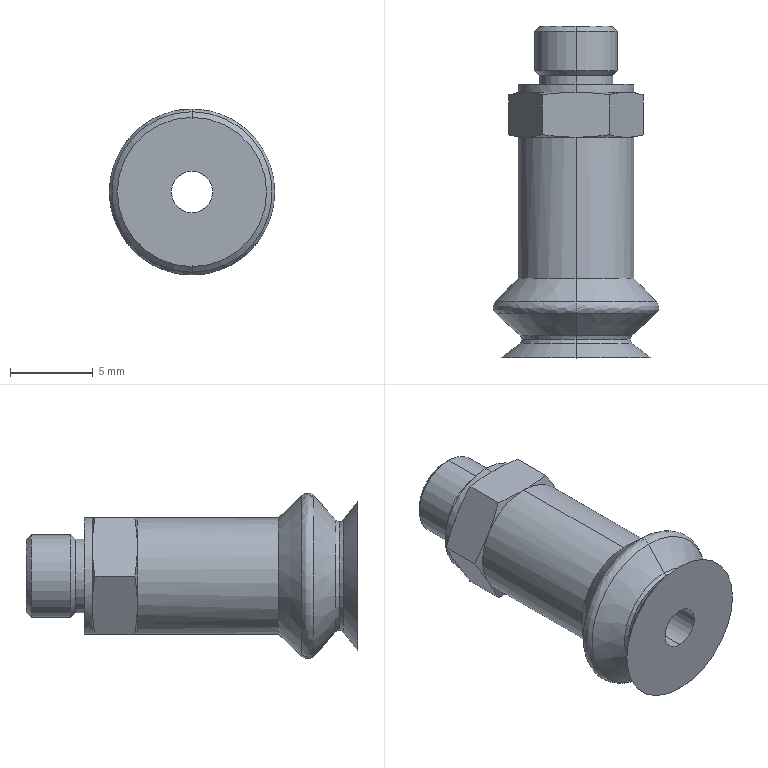Part | SolidWorks | features BaseBody 1 | 1 solid | 48 faces | box 9.996 x 20 x 10 mm | volume 691.38 mm3 | cone 22 | cylinder 10 | plane 10 | spline 6 | commonest cylinder face diameters 7 x4 2.5 x2 4.46 x2 5 x2
STEP:
#1=CARTESIAN_POINT('',(0.,3.375,4.861));
#2=VERTEX_POINT('',#1);
#3=CARTESIAN_POINT('',(0.,3.375,-4.861));
#4=VERTEX_POINT('',#3);
#5=CARTESIAN_POINT('',(0.,3.375,0.));
#6=DIRECTION('',(0.,-1.,0.));
#7=DIRECTION('',(0.,0.,1.));
#8=AXIS2_PLACEMENT_3D('',#5,#6,#7);
#9=CIRCLE('',#8,4.861);
#10=EDGE_CURVE('',#2,#4,#9,.T.);
#11=ORIENTED_EDGE('',*,*,#10,.T.);
#12=CARTESIAN_POINT('',(0.,2.659,-4.835));
#13=VERTEX_POINT('',#12);
#14=CARTESIAN_POINT('',(0.,3.03,-4.5));
#15=DIRECTION('',(-1.,0.,0.));
#16=DIRECTION('',(0.,0.,1.));
#17=AXIS2_PLACEMENT_3D('',#14,#15,#16);
#18=CIRCLE('',#17,0.5);
#19=EDGE_CURVE('',#4,#13,#18,.T.);
#20=ORIENTED_EDGE('',*,*,#19,.T.);
#21=CARTESIAN_POINT('',(0.,2.659,4.835));
#22=VERTEX_POINT('',#21);
#23=CARTESIAN_POINT('',(0.,2.659,0.));
#24=DIRECTION('',(0.,1.,0.));
#25=DIRECTION('',(0.,0.,1.));
#26=AXIS2_PLACEMENT_3D('',#23,#24,#25);
#27=CIRCLE('',#26,4.835);
#28=EDGE_CURVE('',#13,#22,#27,.T.);
#29=ORIENTED_EDGE('',*,*,#28,.T.);
#30=CARTESIAN_POINT('',(0.,3.03,4.5));
#31=DIRECTION('',(1.,0.,0.));
#32=DIRECTION('',(0.,0.,-1.));
#33=AXIS2_PLACEMENT_3D('',#30,#31,#32);
#34=CIRCLE('',#33,0.5);
#35=EDGE_CURVE('',#2,#22,#34,.T.);
#36=ORIENTED_EDGE('',*,*,#35,.F.);
#37=EDGE_LOOP('',(#11,#20,#29,#36));
#38=FACE_OUTER_BOUND('',#37,.T.);
#39=CARTESIAN_POINT('',(0.,3.375,-4.861));
#40=CARTESIAN_POINT('',(-9.723,3.375,-4.861));
#41=CARTESIAN_POINT('',(-9.723,3.375,4.861));
#42=CARTESIAN_POINT('',(0.,3.375,4.861));
#43=CARTESIAN_POINT('',(0.,3.159,-5.068));
#44=CARTESIAN_POINT('',(-10.137,3.159,-5.068));
#45=CARTESIAN_POINT('',(-10.137,3.159,5.068));
#46=CARTESIAN_POINT('',(0.,3.159,5.068));
#47=CARTESIAN_POINT('',(0.,2.86,-5.057));
#48=CARTESIAN_POINT('',(-10.115,2.86,-5.057));
#49=CARTESIAN_POINT('',(-10.115,2.86,5.057));
#50=CARTESIAN_POINT('',(0.,2.86,5.057));
#51=CARTESIAN_POINT('',(0.,2.659,-4.835));
#52=CARTESIAN_POINT('',(-9.671,2.659,-4.835));
#53=CARTESIAN_POINT('',(-9.671,2.659,4.835));
#54=CARTESIAN_POINT('',(0.,2.659,4.835));
#55=(BOUNDED_SURFACE()B_SPLINE_SURFACE(3,3,((#39,#40,#41,#42),(#43,#44,#45,#46),(#47,#48,#49,#50),(#51,#52,#53,#54)),.UNSPECIFIED.,.F.,.F.,.T.)B_SPLINE_SURFACE_WITH_KNOTS((4,4),(4,4),(0.,1.),(0.,1.),.UNSPECIFIED.)GEOMETRIC_REPRESENTATION_ITEM()RATIONAL_B_SPLINE_SURFACE(((1.,0.3333,0.3333,1.),(0.7982,0.2661,0.2661,0.7982),(0.7982,0.2661,0.2661,0.7982),(1.,0.3333,0.3333,1.)))REPRESENTATION_ITEM('')SURFACE());
#56=ADVANCED_FACE('',(#38),#55,.T.);
#57=CARTESIAN_POINT('',(0.,1.11,-3.27));
#58=VERTEX_POINT('',#57);
#59=CARTESIAN_POINT('',(0.,1.11,3.27));
#60=VERTEX_POINT('',#59);
#61=CARTESIAN_POINT('',(0.,1.11,0.));
#62=DIRECTION('',(0.,1.,0.));
#63=DIRECTION('',(0.,0.,1.));
#64=AXIS2_PLACEMENT_3D('',#61,#62,#63);
#65=CIRCLE('',#64,3.27);
#66=EDGE_CURVE('',#58,#60,#65,.T.);
#67=ORIENTED_EDGE('',*,*,#66,.F.);
#68=CARTESIAN_POINT('',(0.,0.8739,-3.385));
#69=VERTEX_POINT('',#68);
#70=CARTESIAN_POINT('',(0.,1.11,-3.57));
#71=DIRECTION('',(1.,0.,0.));
#72=DIRECTION('',(0.,0.,1.));
#73=AXIS2_PLACEMENT_3D('',#70,#71,#72);
#74=CIRCLE('',#73,0.3);
#75=EDGE_CURVE('',#58,#69,#74,.T.);
#76=ORIENTED_EDGE('',*,*,#75,.T.);
#77=CARTESIAN_POINT('',(0.,0.8739,3.385));
#78=VERTEX_POINT('',#77);
#79=CARTESIAN_POINT('',(0.,0.8739,0.));
#80=DIRECTION('',(0.,1.,0.));
#81=DIRECTION('',(0.,0.,1.));
#82=AXIS2_PLACEMENT_3D('',#79,#80,#81);
#83=CIRCLE('',#82,3.385);
#84=EDGE_CURVE('',#69,#78,#83,.T.);
#85=ORIENTED_EDGE('',*,*,#84,.T.);
#86=CARTESIAN_POINT('',(0.,1.11,3.57));
#87=DIRECTION('',(-1.,0.,0.));
#88=DIRECTION('',(0.,0.,-1.));
#89=AXIS2_PLACEMENT_3D('',#86,#87,#88);
#90=CIRCLE('',#89,0.3);
#91=EDGE_CURVE('',#60,#78,#90,.T.);
#92=ORIENTED_EDGE('',*,*,#91,.F.);
#93=EDGE_LOOP('',(#67,#76,#85,#92));
#94=FACE_OUTER_BOUND('',#93,.T.);
#95=CARTESIAN_POINT('',(0.,1.11,-3.27));
#96=CARTESIAN_POINT('',(-6.54,1.11,-3.27));
#97=CARTESIAN_POINT('',(-6.54,1.11,3.27));
#98=CARTESIAN_POINT('',(0.,1.11,3.27));
#99=CARTESIAN_POINT('',(0.,1.016,-3.27));
#100=CARTESIAN_POINT('',(-6.54,1.016,-3.27));
#101=CARTESIAN_POINT('',(-6.54,1.016,3.27));
#102=CARTESIAN_POINT('',(0.,1.016,3.27));
#103=CARTESIAN_POINT('',(0.,0.9318,-3.311));
#104=CARTESIAN_POINT('',(-6.622,0.9318,-3.311));
#105=CARTESIAN_POINT('',(-6.622,0.9318,3.311));
#106=CARTESIAN_POINT('',(0.,0.9318,3.311));
#107=CARTESIAN_POINT('',(0.,0.8739,-3.385));
#108=CARTESIAN_POINT('',(-6.77,0.8739,-3.385));
#109=CARTESIAN_POINT('',(-6.77,0.8739,3.385));
#110=CARTESIAN_POINT('',(0.,0.8739,3.385));
#111=(BOUNDED_SURFACE()B_SPLINE_SURFACE(3,3,((#95,#96,#97,#98),(#99,#100,#101,#102),(#103,#104,#105,#106),(#107,#108,#109,#110)),.UNSPECIFIED.,.F.,.F.,.T.)B_SPLINE_SURFACE_WITH_KNOTS((4,4),(4,4),(0.,1.),(0.,1.),.UNSPECIFIED.)GEOMETRIC_REPRESENTATION_ITEM()RATIONAL_B_SPLINE_SURFACE(((1.,0.3333,0.3333,1.),(0.9327,0.3109,0.3109,0.9327),(0.9327,0.3109,0.3109,0.9327),(1.,0.3333,0.3333,1.)))REPRESENTATION_ITEM('')SURFACE());
#112=ADVANCED_FACE('',(#94),#111,.T.);
#113=CARTESIAN_POINT('',(0.,1.332,-3.369));
#114=VERTEX_POINT('',#113);
#115=CARTESIAN_POINT('',(0.,1.332,3.369));
#116=VERTEX_POINT('',#115);
#117=CARTESIAN_POINT('',(0.,1.332,0.));
#118=DIRECTION('',(0.,1.,0.));
#119=DIRECTION('',(1.,0.,0.));
#120=AXIS2_PLACEMENT_3D('',#117,#118,#119);
#121=CIRCLE('',#120,3.369);
#122=EDGE_CURVE('',#114,#116,#121,.T.);
#123=ORIENTED_EDGE('',*,*,#122,.F.);
#124=CARTESIAN_POINT('',(0.,1.11,-3.57));
#125=DIRECTION('',(1.,0.,0.));
#126=DIRECTION('',(0.,0.,1.));
#127=AXIS2_PLACEMENT_3D('',#124,#125,#126);
#128=CIRCLE('',#127,0.3);
#129=EDGE_CURVE('',#114,#58,#128,.T.);
#130=ORIENTED_EDGE('',*,*,#129,.T.);
#131=ORIENTED_EDGE('',*,*,#66,.T.);
#132=CARTESIAN_POINT('',(0.,1.11,3.57));
#133=DIRECTION('',(-1.,0.,0.));
#134=DIRECTION('',(0.,0.,-1.));
#135=AXIS2_PLACEMENT_3D('',#132,#133,#134);
#136=CIRCLE('',#135,0.3);
#137=EDGE_CURVE('',#116,#60,#136,.T.);
#138=ORIENTED_EDGE('',*,*,#137,.F.);
#139=EDGE_LOOP('',(#123,#130,#131,#138));
#140=FACE_OUTER_BOUND('',#139,.T.);
#141=CARTESIAN_POINT('',(0.,1.332,-3.369));
#142=CARTESIAN_POINT('',(-6.737,1.332,-3.369));
#143=CARTESIAN_POINT('',(-6.737,1.332,3.369));
#144=CARTESIAN_POINT('',(0.,1.332,3.369));
#145=CARTESIAN_POINT('',(0.,1.275,-3.305));
#146=CARTESIAN_POINT('',(-6.61,1.275,-3.305));
#147=CARTESIAN_POINT('',(-6.61,1.275,3.305));
#148=CARTESIAN_POINT('',(0.,1.275,3.305));
#149=CARTESIAN_POINT('',(0.,1.196,-3.27));
#150=CARTESIAN_POINT('',(-6.54,1.196,-3.27));
#151=CARTESIAN_POINT('',(-6.54,1.196,3.27));
#152=CARTESIAN_POINT('',(0.,1.196,3.27));
#153=CARTESIAN_POINT('',(0.,1.11,-3.27));
#154=CARTESIAN_POINT('',(-6.54,1.11,-3.27));
#155=CARTESIAN_POINT('',(-6.54,1.11,3.27));
#156=CARTESIAN_POINT('',(0.,1.11,3.27));
#157=(BOUNDED_SURFACE()B_SPLINE_SURFACE(3,3,((#141,#142,#143,#144),(#145,#146,#147,#148),(#149,#150,#151,#152),(#153,#154,#155,#156)),.UNSPECIFIED.,.F.,.F.,.F.)B_SPLINE_SURFACE_WITH_KNOTS((4,4),(4,4),(0.,1.),(0.,1.),.UNSPECIFIED.)GEOMETRIC_REPRESENTATION_ITEM()RATIONAL_B_SPLINE_SURFACE(((1.,0.3333,0.3333,1.),(0.9427,0.3142,0.3142,0.9427),(0.9427,0.3142,0.3142,0.9427),(1.,0.3333,0.3333,1.)))REPRESENTATION_ITEM('')SURFACE());
#158=ADVANCED_FACE('',(#140),#157,.T.);
#159=CARTESIAN_POINT('',(0.,1.332,0.));
#160=DIRECTION('',(0.,1.,0.));
#161=DIRECTION('',(1.,0.,0.));
#162=AXIS2_PLACEMENT_3D('',#159,#160,#161);
#163=CIRCLE('',#162,3.369);
#164=EDGE_CURVE('',#116,#114,#163,.T.);
#165=ORIENTED_EDGE('',*,*,#164,.T.);
#166=CARTESIAN_POINT('',(0.,1.332,-3.369));
#167=DIRECTION('',(0.,0.6708,-0.7416));
#168=VECTOR('',#167,1000.);
#169=LINE('',#166,#168);
#170=EDGE_CURVE('',#114,#13,#169,.T.);
#171=ORIENTED_EDGE('',*,*,#170,.T.);
#172=CARTESIAN_POINT('',(0.,2.659,0.));
#173=DIRECTION('',(0.,1.,0.));
#174=DIRECTION('',(0.,0.,1.));
#175=AXIS2_PLACEMENT_3D('',#172,#173,#174);
#176=CIRCLE('',#175,4.835);
#177=EDGE_CURVE('',#22,#13,#176,.T.);
#178=ORIENTED_EDGE('',*,*,#177,.F.);
#179=CARTESIAN_POINT('',(0.,1.332,3.369));
#180=DIRECTION('',(0.,0.6708,0.7416));
#181=VECTOR('',#180,1000.);
#182=LINE('',#179,#181);
#183=EDGE_CURVE('',#116,#22,#182,.T.);
#184=ORIENTED_EDGE('',*,*,#183,.F.);
#185=EDGE_LOOP('',(#165,#171,#178,#184));
#186=FACE_OUTER_BOUND('',#185,.T.);
#187=CARTESIAN_POINT('',(0.,1.332,0.));
#188=DIRECTION('',(0.,1.,0.));
#189=DIRECTION('',(0.,0.,1.));
#190=AXIS2_PLACEMENT_3D('',#187,#188,#189);
#191=CONICAL_SURFACE('',#190,3.369,0.8355);
#192=ADVANCED_FACE('',(#186),#191,.T.);
#193=ORIENTED_EDGE('',*,*,#129,.F.);
#194=ORIENTED_EDGE('',*,*,#164,.F.);
#195=ORIENTED_EDGE('',*,*,#137,.T.);
#196=CARTESIAN_POINT('',(0.,1.11,0.));
#197=DIRECTION('',(0.,1.,0.));
#198=DIRECTION('',(0.,0.,1.));
#199=AXIS2_PLACEMENT_3D('',#196,#197,#198);
#200=CIRCLE('',#199,3.27);
#201=EDGE_CURVE('',#60,#58,#200,.T.);
#202=ORIENTED_EDGE('',*,*,#201,.T.);
#203=EDGE_LOOP('',(#193,#194,#195,#202));
#204=FACE_OUTER_BOUND('',#203,.T.);
#205=CARTESIAN_POINT('',(0.,1.332,3.369));
#206=CARTESIAN_POINT('',(6.737,1.332,3.369));
#207=CARTESIAN_POINT('',(6.737,1.332,-3.369));
#208=CARTESIAN_POINT('',(0.,1.332,-3.369));
#209=CARTESIAN_POINT('',(0.,1.275,3.305));
#210=CARTESIAN_POINT('',(6.61,1.275,3.305));
#211=CARTESIAN_POINT('',(6.61,1.275,-3.305));
#212=CARTESIAN_POINT('',(0.,1.275,-3.305));
#213=CARTESIAN_POINT('',(0.,1.196,3.27));
#214=CARTESIAN_POINT('',(6.54,1.196,3.27));
#215=CARTESIAN_POINT('',(6.54,1.196,-3.27));
#216=CARTESIAN_POINT('',(0.,1.196,-3.27));
#217=CARTESIAN_POINT('',(0.,1.11,3.27));
#218=CARTESIAN_POINT('',(6.54,1.11,3.27));
#219=CARTESIAN_POINT('',(6.54,1.11,-3.27));
#220=CARTESIAN_POINT('',(0.,1.11,-3.27));
#221=(BOUNDED_SURFACE()B_SPLINE_SURFACE(3,3,((#205,#206,#207,#208),(#209,#210,#211,#212),(#213,#214,#215,#216),(#217,#218,#219,#220)),.UNSPECIFIED.,.F.,.F.,.F.)B_SPLINE_SURFACE_WITH_KNOTS((4,4),(4,4),(0.,1.),(0.,1.),.UNSPECIFIED.)GEOMETRIC_REPRESENTATION_ITEM()RATIONAL_B_SPLINE_SURFACE(((1.,0.3333,0.3333,1.),(0.9427,0.3142,0.3142,0.9427),(0.9427,0.3142,0.3142,0.9427),(1.,0.3333,0.3333,1.)))REPRESENTATION_ITEM('')SURFACE());
#222=ADVANCED_FACE('',(#204),#221,.T.);
#223=CARTESIAN_POINT('',(0.,4.8,-3.5));
#224=VERTEX_POINT('',#223);
#225=CARTESIAN_POINT('',(0.,4.8,3.5));
#226=VERTEX_POINT('',#225);
#227=CARTESIAN_POINT('',(0.,4.8,0.));
#228=DIRECTION('',(0.,-1.,0.));
#229=DIRECTION('',(1.,0.,0.));
#230=AXIS2_PLACEMENT_3D('',#227,#228,#229);
#231=CIRCLE('',#230,3.5);
#232=EDGE_CURVE('',#224,#226,#231,.T.);
#233=ORIENTED_EDGE('',*,*,#232,.T.);
#234=CARTESIAN_POINT('',(0.,4.8,3.5));
#235=DIRECTION('',(0.,-0.7229,0.6909));
#236=VECTOR('',#235,1000.);
#237=LINE('',#234,#236);
#238=EDGE_CURVE('',#226,#2,#237,.T.);
#239=ORIENTED_EDGE('',*,*,#238,.T.);
#240=CARTESIAN_POINT('',(0.,3.375,0.));
#241=DIRECTION('',(0.,-1.,0.));
#242=DIRECTION('',(0.,0.,1.));
#243=AXIS2_PLACEMENT_3D('',#240,#241,#242);
#244=CIRCLE('',#243,4.861);
#245=EDGE_CURVE('',#4,#2,#244,.T.);
#246=ORIENTED_EDGE('',*,*,#245,.F.);
#247=CARTESIAN_POINT('',(0.,4.8,-3.5));
#248=DIRECTION('',(0.,-0.7229,-0.6909));
#249=VECTOR('',#248,1000.);
#250=LINE('',#247,#249);
#251=EDGE_CURVE('',#224,#4,#250,.T.);
#252=ORIENTED_EDGE('',*,*,#251,.F.);
#253=EDGE_LOOP('',(#233,#239,#246,#252));
#254=FACE_OUTER_BOUND('',#253,.T.);
#255=CARTESIAN_POINT('',(0.,4.8,0.));
#256=DIRECTION('',(0.,-1.,0.));
#257=DIRECTION('',(0.,0.,-1.));
#258=AXIS2_PLACEMENT_3D('',#255,#256,#257);
#259=CONICAL_SURFACE('',#258,3.5,0.7628);
#260=ADVANCED_FACE('',(#254),#259,.T.);
#261=ORIENTED_EDGE('',*,*,#232,.F.);
#262=CARTESIAN_POINT('',(0.,13.3,-3.5));
#263=VERTEX_POINT('',#262);
#264=CARTESIAN_POINT('',(0.,13.,-3.5));
#265=DIRECTION('',(0.,1.,0.));
#266=VECTOR('',#265,1000.);
#267=LINE('',#264,#266);
#268=EDGE_CURVE('',#224,#263,#267,.T.);
#269=ORIENTED_EDGE('',*,*,#268,.T.);
#270=CARTESIAN_POINT('',(3.031,13.3,-1.75));
#271=VERTEX_POINT('',#270);
#272=CARTESIAN_POINT('',(0.,13.3,0.));
#273=DIRECTION('',(0.,-1.,0.));
#274=DIRECTION('',(1.,0.,0.));
#275=AXIS2_PLACEMENT_3D('',#272,#273,#274);
#276=CIRCLE('',#275,3.5);
#277=EDGE_CURVE('',#263,#271,#276,.T.);
#278=ORIENTED_EDGE('',*,*,#277,.T.);
#279=CARTESIAN_POINT('',(3.031,13.3,1.75));
#280=VERTEX_POINT('',#279);
#281=CARTESIAN_POINT('',(0.,13.3,0.));
#282=DIRECTION('',(0.,-1.,0.));
#283=DIRECTION('',(1.,0.,0.));
#284=AXIS2_PLACEMENT_3D('',#281,#282,#283);
#285=CIRCLE('',#284,3.5);
#286=EDGE_CURVE('',#271,#280,#285,.T.);
#287=ORIENTED_EDGE('',*,*,#286,.T.);
#288=CARTESIAN_POINT('',(0.,13.3,3.5));
#289=VERTEX_POINT('',#288);
#290=CARTESIAN_POINT('',(0.,13.3,0.));
#291=DIRECTION('',(0.,-1.,0.));
#292=DIRECTION('',(1.,0.,0.));
#293=AXIS2_PLACEMENT_3D('',#290,#291,#292);
#294=CIRCLE('',#293,3.5);
#295=EDGE_CURVE('',#280,#289,#294,.T.);
#296=ORIENTED_EDGE('',*,*,#295,.T.);
#297=CARTESIAN_POINT('',(0.,13.,3.5));
#298=DIRECTION('',(0.,1.,0.));
#299=VECTOR('',#298,1000.);
#300=LINE('',#297,#299);
#301=EDGE_CURVE('',#226,#289,#300,.T.);
#302=ORIENTED_EDGE('',*,*,#301,.F.);
#303=EDGE_LOOP('',(#261,#269,#278,#287,#296,#302));
#304=FACE_OUTER_BOUND('',#303,.T.);
#305=CARTESIAN_POINT('',(0.,13.,0.));
#306=DIRECTION('',(0.,1.,0.));
#307=DIRECTION('',(0.,0.,1.));
#308=AXIS2_PLACEMENT_3D('',#305,#306,#307);
#309=CYLINDRICAL_SURFACE('',#308,3.5);
#310=ADVANCED_FACE('',(#304),#309,.T.);
#311=CARTESIAN_POINT('',(0.,0.8739,0.));
#312=DIRECTION('',(0.,1.,0.));
#313=DIRECTION('',(0.,0.,1.));
#314=AXIS2_PLACEMENT_3D('',#311,#312,#313);
#315=CIRCLE('',#314,3.385);
#316=EDGE_CURVE('',#78,#69,#315,.T.);
#317=ORIENTED_EDGE('',*,*,#316,.F.);
#318=CARTESIAN_POINT('',(0.,0.,4.5));
#319=VERTEX_POINT('',#318);
#320=CARTESIAN_POINT('',(0.,0.8739,3.385));
#321=DIRECTION('',(0.,-0.6168,0.7871));
#322=VECTOR('',#321,1000.);
#323=LINE('',#320,#322);
#324=EDGE_CURVE('',#78,#319,#323,.T.);
#325=ORIENTED_EDGE('',*,*,#324,.T.);
#326=CARTESIAN_POINT('',(0.,0.,-4.5));
#327=VERTEX_POINT('',#326);
#328=CARTESIAN_POINT('',(0.,0.,0.));
#329=DIRECTION('',(0.,1.,0.));
#330=DIRECTION('',(0.,0.,-1.));
#331=AXIS2_PLACEMENT_3D('',#328,#329,#330);
#332=CIRCLE('',#331,4.5);
#333=EDGE_CURVE('',#319,#327,#332,.T.);
#334=ORIENTED_EDGE('',*,*,#333,.T.);
#335=CARTESIAN_POINT('',(0.,0.8739,-3.385));
#336=DIRECTION('',(0.,-0.6168,-0.7871));
#337=VECTOR('',#336,1000.);
#338=LINE('',#335,#337);
#339=EDGE_CURVE('',#69,#327,#338,.T.);
#340=ORIENTED_EDGE('',*,*,#339,.F.);
#341=EDGE_LOOP('',(#317,#325,#334,#340));
#342=FACE_OUTER_BOUND('',#341,.T.);
#343=CARTESIAN_POINT('',(0.,0.8739,0.));
#344=DIRECTION('',(0.,-1.,0.));
#345=DIRECTION('',(0.,0.,-1.));
#346=AXIS2_PLACEMENT_3D('',#343,#344,#345);
#347=CONICAL_SURFACE('',#346,3.385,0.9061);
#348=ADVANCED_FACE('',(#342),#347,.T.);
#349=CARTESIAN_POINT('',(0.,0.,-1.25));
#350=VERTEX_POINT('',#349);
#351=CARTESIAN_POINT('',(0.,0.,1.25));
#352=VERTEX_POINT('',#351);
#353=CARTESIAN_POINT('',(0.,0.,0.));
#354=DIRECTION('',(0.,1.,0.));
#355=DIRECTION('',(0.,0.,1.));
#356=AXIS2_PLACEMENT_3D('',#353,#354,#355);
#357=CIRCLE('',#356,1.25);
#358=EDGE_CURVE('',#350,#352,#357,.T.);
#359=ORIENTED_EDGE('',*,*,#358,.F.);
#360=CARTESIAN_POINT('',(0.,20.,-1.25));
#361=VERTEX_POINT('',#360);
#362=CARTESIAN_POINT('',(0.,0.,-1.25));
#363=DIRECTION('',(0.,1.,0.));
#364=VECTOR('',#363,1000.);
#365=LINE('',#362,#364);
#366=EDGE_CURVE('',#350,#361,#365,.T.);
#367=ORIENTED_EDGE('',*,*,#366,.T.);
#368=CARTESIAN_POINT('',(0.,20.,1.25));
#369=VERTEX_POINT('',#368);
#370=CARTESIAN_POINT('',(0.,20.,0.));
#371=DIRECTION('',(0.,1.,0.));
#372=DIRECTION('',(0.,0.,1.));
#373=AXIS2_PLACEMENT_3D('',#370,#371,#372);
#374=CIRCLE('',#373,1.25);
#375=EDGE_CURVE('',#361,#369,#374,.T.);
#376=ORIENTED_EDGE('',*,*,#375,.T.);
#377=CARTESIAN_POINT('',(0.,0.,1.25));
#378=DIRECTION('',(0.,1.,0.));
#379=VECTOR('',#378,1000.);
#380=LINE('',#377,#379);
#381=EDGE_CURVE('',#352,#369,#380,.T.);
#382=ORIENTED_EDGE('',*,*,#381,.F.);
#383=EDGE_LOOP('',(#359,#367,#376,#382));
#384=FACE_OUTER_BOUND('',#383,.T.);
#385=CARTESIAN_POINT('',(0.,0.,0.));
#386=DIRECTION('',(0.,1.,0.));
#387=DIRECTION('',(0.,0.,1.));
#388=AXIS2_PLACEMENT_3D('',#385,#386,#387);
#389=CYLINDRICAL_SURFACE('',#388,1.25);
#390=ADVANCED_FACE('',(#384),#389,.F.);
#391=CARTESIAN_POINT('',(0.,16.,-3.5));
#392=VERTEX_POINT('',#391);
#393=CARTESIAN_POINT('',(3.031,16.,-1.75));
#394=VERTEX_POINT('',#393);
#395=CARTESIAN_POINT('',(0.,16.,0.));
#396=DIRECTION('',(0.,-1.,0.));
#397=DIRECTION('',(1.,0.,0.));
#398=AXIS2_PLACEMENT_3D('',#395,#396,#397);
#399=CIRCLE('',#398,3.5);
#400=EDGE_CURVE('',#392,#394,#399,.T.);
#401=ORIENTED_EDGE('',*,*,#400,.F.);
#402=CARTESIAN_POINT('',(0.,16.5,-3.5));
#403=VERTEX_POINT('',#402);
#404=CARTESIAN_POINT('',(0.,16.5,-3.5));
#405=DIRECTION('',(0.,1.,0.));
#406=VECTOR('',#405,1000.);
#407=LINE('',#404,#406);
#408=EDGE_CURVE('',#392,#403,#407,.T.);
#409=ORIENTED_EDGE('',*,*,#408,.T.);
#410=CARTESIAN_POINT('',(0.,16.5,3.5));
#411=VERTEX_POINT('',#410);
#412=CARTESIAN_POINT('',(0.,16.5,0.));
#413=DIRECTION('',(0.,-1.,0.));
#414=DIRECTION('',(0.,0.,1.));
#415=AXIS2_PLACEMENT_3D('',#412,#413,#414);
#416=CIRCLE('',#415,3.5);
#417=EDGE_CURVE('',#403,#411,#416,.T.);
#418=ORIENTED_EDGE('',*,*,#417,.T.);
#419=CARTESIAN_POINT('',(0.,16.,3.5));
#420=VERTEX_POINT('',#419);
#421=CARTESIAN_POINT('',(0.,16.5,3.5));
#422=DIRECTION('',(0.,1.,0.));
#423=VECTOR('',#422,1000.);
#424=LINE('',#421,#423);
#425=EDGE_CURVE('',#420,#411,#424,.T.);
#426=ORIENTED_EDGE('',*,*,#425,.F.);
#427=CARTESIAN_POINT('',(3.031,16.,1.75));
#428=VERTEX_POINT('',#427);
#429=CARTESIAN_POINT('',(0.,16.,0.));
#430=DIRECTION('',(0.,-1.,0.));
#431=DIRECTION('',(1.,0.,0.));
#432=AXIS2_PLACEMENT_3D('',#429,#430,#431);
#433=CIRCLE('',#432,3.5);
#434=EDGE_CURVE('',#428,#420,#433,.T.);
#435=ORIENTED_EDGE('',*,*,#434,.F.);
#436=CARTESIAN_POINT('',(0.,16.,0.));
#437=DIRECTION('',(0.,-1.,0.));
#438=DIRECTION('',(1.,0.,0.));
#439=AXIS2_PLACEMENT_3D('',#436,#437,#438);
#440=CIRCLE('',#439,3.5);
#441=EDGE_CURVE('',#394,#428,#440,.T.);
#442=ORIENTED_EDGE('',*,*,#441,.F.);
#443=EDGE_LOOP('',(#401,#409,#418,#426,#435,#442));
#444=FACE_OUTER_BOUND('',#443,.T.);
#445=CARTESIAN_POINT('',(0.,16.5,0.));
#446=DIRECTION('',(0.,1.,0.));
#447=DIRECTION('',(0.,0.,1.));
#448=AXIS2_PLACEMENT_3D('',#445,#446,#447);
#449=CYLINDRICAL_SURFACE('',#448,3.5);
#450=ADVANCED_FACE('',(#444),#449,.T.);
#451=CARTESIAN_POINT('',(0.,20.,2.193));
#452=VERTEX_POINT('',#451);
#453=CARTESIAN_POINT('',(0.,20.,-2.193));
#454=VERTEX_POINT('',#453);
#455=CARTESIAN_POINT('',(0.,20.,0.));
#456=DIRECTION('',(0.,1.,0.));
#457=DIRECTION('',(0.,0.,-1.));
#458=AXIS2_PLACEMENT_3D('',#455,#456,#457);
#459=CIRCLE('',#458,2.193);
#460=EDGE_CURVE('',#452,#454,#459,.T.);
#461=ORIENTED_EDGE('',*,*,#460,.F.);
#462=CARTESIAN_POINT('',(0.,19.694,2.5));
#463=VERTEX_POINT('',#462);
#464=CARTESIAN_POINT('',(0.,20.,2.194));
#465=DIRECTION('',(0.,-0.7071,0.7071));
#466=VECTOR('',#465,1000.);
#467=LINE('',#464,#466);
#468=EDGE_CURVE('',#452,#463,#467,.T.);
#469=ORIENTED_EDGE('',*,*,#468,.T.);
#470=CARTESIAN_POINT('',(0.,19.694,-2.5));
#471=VERTEX_POINT('',#470);
#472=CARTESIAN_POINT('',(0.,19.694,0.));
#473=DIRECTION('',(0.,1.,0.));
#474=DIRECTION('',(1.,0.,0.));
#475=AXIS2_PLACEMENT_3D('',#472,#473,#474);
#476=CIRCLE('',#475,2.5);
#477=EDGE_CURVE('',#463,#471,#476,.T.);
#478=ORIENTED_EDGE('',*,*,#477,.T.);
#479=CARTESIAN_POINT('',(0.,20.,-2.194));
#480=DIRECTION('',(0.,-0.7071,-0.7071));
#481=VECTOR('',#480,1000.);
#482=LINE('',#479,#481);
#483=EDGE_CURVE('',#454,#471,#482,.T.);
#484=ORIENTED_EDGE('',*,*,#483,.F.);
#485=EDGE_LOOP('',(#461,#469,#478,#484));
#486=FACE_OUTER_BOUND('',#485,.T.);
#487=CARTESIAN_POINT('',(0.,20.,0.));
#488=DIRECTION('',(0.,-1.,0.));
#489=DIRECTION('',(0.,0.,-1.));
#490=AXIS2_PLACEMENT_3D('',#487,#488,#489);
#491=CONICAL_SURFACE('',#490,2.194,0.7854);
#492=ADVANCED_FACE('',(#486),#491,.T.);
#493=CARTESIAN_POINT('',(0.,17.306,2.5));
#494=VERTEX_POINT('',#493);
#495=CARTESIAN_POINT('',(0.,17.306,-2.5));
#496=VERTEX_POINT('',#495);
#497=CARTESIAN_POINT('',(0.,17.306,0.));
#498=DIRECTION('',(0.,1.,0.));
#499=DIRECTION('',(1.,0.,0.));
#500=AXIS2_PLACEMENT_3D('',#497,#498,#499);
#501=CIRCLE('',#500,2.5);
#502=EDGE_CURVE('',#494,#496,#501,.T.);
#503=ORIENTED_EDGE('',*,*,#502,.T.);
#504=CARTESIAN_POINT('',(0.,19.694,-2.5));
#505=DIRECTION('',(0.,1.,0.));
#506=VECTOR('',#505,1000.);
#507=LINE('',#504,#506);
#508=EDGE_CURVE('',#496,#471,#507,.T.);
#509=ORIENTED_EDGE('',*,*,#508,.T.);
#510=ORIENTED_EDGE('',*,*,#477,.F.);
#511=CARTESIAN_POINT('',(0.,19.694,2.5));
#512=DIRECTION('',(0.,1.,0.));
#513=VECTOR('',#512,1000.);
#514=LINE('',#511,#513);
#515=EDGE_CURVE('',#494,#463,#514,.T.);
#516=ORIENTED_EDGE('',*,*,#515,.F.);
#517=EDGE_LOOP('',(#503,#509,#510,#516));
#518=FACE_OUTER_BOUND('',#517,.T.);
#519=CARTESIAN_POINT('',(0.,19.694,0.));
#520=DIRECTION('',(0.,1.,0.));
#521=DIRECTION('',(0.,0.,1.));
#522=AXIS2_PLACEMENT_3D('',#519,#520,#521);
#523=CYLINDRICAL_SURFACE('',#522,2.5);
#524=ADVANCED_FACE('',(#518),#523,.T.);
#525=CARTESIAN_POINT('',(0.,16.5,-2.23));
#526=VERTEX_POINT('',#525);
#527=CARTESIAN_POINT('',(0.,16.5,2.23));
#528=VERTEX_POINT('',#527);
#529=CARTESIAN_POINT('',(0.,16.5,0.));
#530=DIRECTION('',(0.,-1.,0.));
#531=DIRECTION('',(0.,0.,1.));
#532=AXIS2_PLACEMENT_3D('',#529,#530,#531);
#533=CIRCLE('',#532,2.23);
#534=EDGE_CURVE('',#526,#528,#533,.T.);
#535=ORIENTED_EDGE('',*,*,#534,.F.);
#536=CARTESIAN_POINT('',(0.,17.,-2.23));
#537=VERTEX_POINT('',#536);
#538=CARTESIAN_POINT('',(0.,17.,-2.23));
#539=DIRECTION('',(0.,1.,0.));
#540=VECTOR('',#539,1000.);
#541=LINE('',#538,#540);
#542=EDGE_CURVE('',#526,#537,#541,.T.);
#543=ORIENTED_EDGE('',*,*,#542,.T.);
#544=CARTESIAN_POINT('',(0.,17.,2.23));
#545=VERTEX_POINT('',#544);
#546=CARTESIAN_POINT('',(0.,17.,0.));
#547=DIRECTION('',(0.,-1.,0.));
#548=DIRECTION('',(0.,0.,1.));
#549=AXIS2_PLACEMENT_3D('',#546,#547,#548);
#550=CIRCLE('',#549,2.23);
#551=EDGE_CURVE('',#537,#545,#550,.T.);
#552=ORIENTED_EDGE('',*,*,#551,.T.);
#553=CARTESIAN_POINT('',(0.,17.,2.23));
#554=DIRECTION('',(0.,1.,0.));
#555=VECTOR('',#554,1000.);
#556=LINE('',#553,#555);
#557=EDGE_CURVE('',#528,#545,#556,.T.);
#558=ORIENTED_EDGE('',*,*,#557,.F.);
#559=EDGE_LOOP('',(#535,#543,#552,#558));
#560=FACE_OUTER_BOUND('',#559,.T.);
#561=CARTESIAN_POINT('',(0.,17.,0.));
#562=DIRECTION('',(0.,1.,0.));
#563=DIRECTION('',(0.,0.,1.));
#564=AXIS2_PLACEMENT_3D('',#561,#562,#563);
#565=CYLINDRICAL_SURFACE('',#564,2.23);
#566=ADVANCED_FACE('',(#560),#565,.T.);
#567=CARTESIAN_POINT('',(0.,17.,2.194));
#568=VERTEX_POINT('',#567);
#569=CARTESIAN_POINT('',(0.,17.,-2.194));
#570=VERTEX_POINT('',#569);
#571=CARTESIAN_POINT('',(0.,17.,0.));
#572=DIRECTION('',(0.,1.,0.));
#573=DIRECTION('',(0.,0.,1.));
#574=AXIS2_PLACEMENT_3D('',#571,#572,#573);
#575=CIRCLE('',#574,2.194);
#576=EDGE_CURVE('',#568,#570,#575,.T.);
#577=ORIENTED_EDGE('',*,*,#576,.T.);
#578=CARTESIAN_POINT('',(0.,17.,-2.194));
#579=DIRECTION('',(0.,0.7071,-0.7071));
#580=VECTOR('',#579,1000.);
#581=LINE('',#578,#580);
#582=EDGE_CURVE('',#570,#496,#581,.T.);
#583=ORIENTED_EDGE('',*,*,#582,.T.);
#584=ORIENTED_EDGE('',*,*,#502,.F.);
#585=CARTESIAN_POINT('',(0.,17.,2.194));
#586=DIRECTION('',(0.,0.7071,0.7071));
#587=VECTOR('',#586,1000.);
#588=LINE('',#585,#587);
#589=EDGE_CURVE('',#568,#494,#588,.T.);
#590=ORIENTED_EDGE('',*,*,#589,.F.);
#591=EDGE_LOOP('',(#577,#583,#584,#590));
#592=FACE_OUTER_BOUND('',#591,.T.);
#593=CARTESIAN_POINT('',(0.,17.,0.));
#594=DIRECTION('',(0.,1.,0.));
#595=DIRECTION('',(0.,0.,1.));
#596=AXIS2_PLACEMENT_3D('',#593,#594,#595);
#597=CONICAL_SURFACE('',#596,2.194,0.7854);
#598=ADVANCED_FACE('',(#592),#597,.T.);
#599=ORIENTED_EDGE('',*,*,#19,.F.);
#600=ORIENTED_EDGE('',*,*,#245,.T.);
#601=ORIENTED_EDGE('',*,*,#35,.T.);
#602=ORIENTED_EDGE('',*,*,#177,.T.);
#603=EDGE_LOOP('',(#599,#600,#601,#602));
#604=FACE_OUTER_BOUND('',#603,.T.);
#605=CARTESIAN_POINT('',(0.,3.375,4.861));
#606=CARTESIAN_POINT('',(9.723,3.375,4.861));
#607=CARTESIAN_POINT('',(9.723,3.375,-4.861));
#608=CARTESIAN_POINT('',(0.,3.375,-4.861));
#609=CARTESIAN_POINT('',(0.,3.159,5.068));
#610=CARTESIAN_POINT('',(10.137,3.159,5.068));
#611=CARTESIAN_POINT('',(10.137,3.159,-5.068));
#612=CARTESIAN_POINT('',(0.,3.159,-5.068));
#613=CARTESIAN_POINT('',(0.,2.86,5.057));
#614=CARTESIAN_POINT('',(10.115,2.86,5.057));
#615=CARTESIAN_POINT('',(10.115,2.86,-5.057));
#616=CARTESIAN_POINT('',(0.,2.86,-5.057));
#617=CARTESIAN_POINT('',(0.,2.659,4.835));
#618=CARTESIAN_POINT('',(9.671,2.659,4.835));
#619=CARTESIAN_POINT('',(9.671,2.659,-4.835));
#620=CARTESIAN_POINT('',(0.,2.659,-4.835));
#621=(BOUNDED_SURFACE()B_SPLINE_SURFACE(3,3,((#605,#606,#607,#608),(#609,#610,#611,#612),(#613,#614,#615,#616),(#617,#618,#619,#620)),.UNSPECIFIED.,.F.,.F.,.F.)B_SPLINE_SURFACE_WITH_KNOTS((4,4),(4,4),(0.,1.),(0.,1.),.UNSPECIFIED.)GEOMETRIC_REPRESENTATION_ITEM()RATIONAL_B_SPLINE_SURFACE(((1.,0.3333,0.3333,1.),(0.7982,0.2661,0.2661,0.7982),(0.7982,0.2661,0.2661,0.7982),(1.,0.3333,0.3333,1.)))REPRESENTATION_ITEM('')SURFACE());
#622=ADVANCED_FACE('',(#604),#621,.T.);
#623=ORIENTED_EDGE('',*,*,#170,.F.);
#624=ORIENTED_EDGE('',*,*,#122,.T.);
#625=ORIENTED_EDGE('',*,*,#183,.T.);
#626=ORIENTED_EDGE('',*,*,#28,.F.);
#627=EDGE_LOOP('',(#623,#624,#625,#626));
#628=FACE_OUTER_BOUND('',#627,.T.);
#629=CARTESIAN_POINT('',(0.,1.332,0.));
#630=DIRECTION('',(0.,1.,0.));
#631=DIRECTION('',(0.,0.,1.));
#632=AXIS2_PLACEMENT_3D('',#629,#630,#631);
#633=CONICAL_SURFACE('',#632,3.369,0.8355);
#634=ADVANCED_FACE('',(#628),#633,.T.);
#635=ORIENTED_EDGE('',*,*,#75,.F.);
#636=ORIENTED_EDGE('',*,*,#201,.F.);
#637=ORIENTED_EDGE('',*,*,#91,.T.);
#638=ORIENTED_EDGE('',*,*,#316,.T.);
#639=EDGE_LOOP('',(#635,#636,#637,#638));
#640=FACE_OUTER_BOUND('',#639,.T.);
#641=CARTESIAN_POINT('',(0.,1.11,3.27));
#642=CARTESIAN_POINT('',(6.54,1.11,3.27));
#643=CARTESIAN_POINT('',(6.54,1.11,-3.27));
#644=CARTESIAN_POINT('',(0.,1.11,-3.27));
#645=CARTESIAN_POINT('',(0.,1.016,3.27));
#646=CARTESIAN_POINT('',(6.54,1.016,3.27));
#647=CARTESIAN_POINT('',(6.54,1.016,-3.27));
#648=CARTESIAN_POINT('',(0.,1.016,-3.27));
#649=CARTESIAN_POINT('',(0.,0.9318,3.311));
#650=CARTESIAN_POINT('',(6.622,0.9318,3.311));
#651=CARTESIAN_POINT('',(6.622,0.9318,-3.311));
#652=CARTESIAN_POINT('',(0.,0.9318,-3.311));
#653=CARTESIAN_POINT('',(0.,0.8739,3.385));
#654=CARTESIAN_POINT('',(6.77,0.8739,3.385));
#655=CARTESIAN_POINT('',(6.77,0.8739,-3.385));
#656=CARTESIAN_POINT('',(0.,0.8739,-3.385));
#657=(BOUNDED_SURFACE()B_SPLINE_SURFACE(3,3,((#641,#642,#643,#644),(#645,#646,#647,#648),(#649,#650,#651,#652),(#653,#654,#655,#656)),.UNSPECIFIED.,.F.,.F.,.F.)B_SPLINE_SURFACE_WITH_KNOTS((4,4),(4,4),(0.,1.),(0.,1.),.UNSPECIFIED.)GEOMETRIC_REPRESENTATION_ITEM()RATIONAL_B_SPLINE_SURFACE(((1.,0.3333,0.3333,1.),(0.9327,0.3109,0.3109,0.9327),(0.9327,0.3109,0.3109,0.9327),(1.,0.3333,0.3333,1.)))REPRESENTATION_ITEM('')SURFACE());
#658=ADVANCED_FACE('',(#640),#657,.T.);
#659=ORIENTED_EDGE('',*,*,#238,.F.);
#660=CARTESIAN_POINT('',(0.,4.8,0.));
#661=DIRECTION('',(0.,-1.,0.));
#662=DIRECTION('',(1.,0.,0.));
#663=AXIS2_PLACEMENT_3D('',#660,#661,#662);
#664=CIRCLE('',#663,3.5);
#665=EDGE_CURVE('',#226,#224,#664,.T.);
#666=ORIENTED_EDGE('',*,*,#665,.T.);
#667=ORIENTED_EDGE('',*,*,#251,.T.);
#668=ORIENTED_EDGE('',*,*,#10,.F.);
#669=EDGE_LOOP('',(#659,#666,#667,#668));
#670=FACE_OUTER_BOUND('',#669,.T.);
#671=CARTESIAN_POINT('',(0.,4.8,0.));
#672=DIRECTION('',(0.,-1.,0.));
#673=DIRECTION('',(0.,0.,-1.));
#674=AXIS2_PLACEMENT_3D('',#671,#672,#673);
#675=CONICAL_SURFACE('',#674,3.5,0.7628);
#676=ADVANCED_FACE('',(#670),#675,.T.);
#677=ORIENTED_EDGE('',*,*,#268,.F.);
#678=ORIENTED_EDGE('',*,*,#665,.F.);
#679=ORIENTED_EDGE('',*,*,#301,.T.);
#680=CARTESIAN_POINT('',(-3.031,13.3,1.75));
#681=VERTEX_POINT('',#680);
#682=CARTESIAN_POINT('',(0.,13.3,0.));
#683=DIRECTION('',(0.,-1.,0.));
#684=DIRECTION('',(1.,0.,0.));
#685=AXIS2_PLACEMENT_3D('',#682,#683,#684);
#686=CIRCLE('',#685,3.5);
#687=EDGE_CURVE('',#289,#681,#686,.T.);
#688=ORIENTED_EDGE('',*,*,#687,.T.);
#689=CARTESIAN_POINT('',(-3.031,13.3,-1.75));
#690=VERTEX_POINT('',#689);
#691=CARTESIAN_POINT('',(0.,13.3,0.));
#692=DIRECTION('',(0.,-1.,0.));
#693=DIRECTION('',(1.,0.,0.));
#694=AXIS2_PLACEMENT_3D('',#691,#692,#693);
#695=CIRCLE('',#694,3.5);
#696=EDGE_CURVE('',#681,#690,#695,.T.);
#697=ORIENTED_EDGE('',*,*,#696,.T.);
#698=CARTESIAN_POINT('',(0.,13.3,0.));
#699=DIRECTION('',(0.,-1.,0.));
#700=DIRECTION('',(1.,0.,0.));
#701=AXIS2_PLACEMENT_3D('',#698,#699,#700);
#702=CIRCLE('',#701,3.5);
#703=EDGE_CURVE('',#690,#263,#702,.T.);
#704=ORIENTED_EDGE('',*,*,#703,.T.);
#705=EDGE_LOOP('',(#677,#678,#679,#688,#697,#704));
#706=FACE_OUTER_BOUND('',#705,.T.);
#707=CARTESIAN_POINT('',(0.,13.,0.));
#708=DIRECTION('',(0.,1.,0.));
#709=DIRECTION('',(0.,0.,1.));
#710=AXIS2_PLACEMENT_3D('',#707,#708,#709);
#711=CYLINDRICAL_SURFACE('',#710,3.5);
#712=ADVANCED_FACE('',(#706),#711,.T.);
#713=ORIENTED_EDGE('',*,*,#324,.F.);
#714=ORIENTED_EDGE('',*,*,#84,.F.);
#715=ORIENTED_EDGE('',*,*,#339,.T.);
#716=CARTESIAN_POINT('',(0.,0.,0.));
#717=DIRECTION('',(0.,1.,0.));
#718=DIRECTION('',(0.,0.,-1.));
#719=AXIS2_PLACEMENT_3D('',#716,#717,#718);
#720=CIRCLE('',#719,4.5);
#721=EDGE_CURVE('',#327,#319,#720,.T.);
#722=ORIENTED_EDGE('',*,*,#721,.T.);
#723=EDGE_LOOP('',(#713,#714,#715,#722));
#724=FACE_OUTER_BOUND('',#723,.T.);
#725=CARTESIAN_POINT('',(0.,0.8739,0.));
#726=DIRECTION('',(0.,-1.,0.));
#727=DIRECTION('',(0.,0.,-1.));
#728=AXIS2_PLACEMENT_3D('',#725,#726,#727);
#729=CONICAL_SURFACE('',#728,3.385,0.9061);
#730=ADVANCED_FACE('',(#724),#729,.T.);
#731=CARTESIAN_POINT('',(0.,0.,0.));
#732=DIRECTION('',(0.,1.,0.));
#733=DIRECTION('',(0.,0.,1.));
#734=AXIS2_PLACEMENT_3D('',#731,#732,#733);
#735=CIRCLE('',#734,1.25);
#736=EDGE_CURVE('',#352,#350,#735,.T.);
#737=ORIENTED_EDGE('',*,*,#736,.T.);
#738=ORIENTED_EDGE('',*,*,#358,.T.);
#739=EDGE_LOOP('',(#737,#738));
#740=FACE_BOUND('',#739,.T.);
#741=ORIENTED_EDGE('',*,*,#721,.F.);
#742=ORIENTED_EDGE('',*,*,#333,.F.);
#743=EDGE_LOOP('',(#741,#742));
#744=FACE_OUTER_BOUND('',#743,.T.);
#745=CARTESIAN_POINT('',(4.5,0.,4.554));
#746=DIRECTION('',(0.,-1.,0.));
#747=DIRECTION('',(-1.,0.,0.));
#748=AXIS2_PLACEMENT_3D('',#745,#746,#747);
#749=PLANE('',#748);
#750=ADVANCED_FACE('',(#740,#744),#749,.T.);
#751=ORIENTED_EDGE('',*,*,#286,.F.);
#752=CARTESIAN_POINT('',(4.041,13.445,0.));
#753=VERTEX_POINT('',#752);
#754=CARTESIAN_POINT('',(3.031,13.3,-1.75));
#755=CARTESIAN_POINT('',(3.37,13.3,-1.164));
#756=CARTESIAN_POINT('',(3.706,13.355,-0.5808));
#757=CARTESIAN_POINT('',(4.041,13.445,0.));
#758=B_SPLINE_CURVE_WITH_KNOTS('',3,(#754,#755,#756,#757),.UNSPECIFIED.,.F.,.F.,(4,4),(0.,0.002026),.UNSPECIFIED.);
#759=EDGE_CURVE('',#271,#753,#758,.T.);
#760=ORIENTED_EDGE('',*,*,#759,.T.);
#761=CARTESIAN_POINT('',(4.041,13.445,0.));
#762=CARTESIAN_POINT('',(3.706,13.355,0.5808));
#763=CARTESIAN_POINT('',(3.37,13.3,1.164));
#764=CARTESIAN_POINT('',(3.031,13.3,1.75));
#765=B_SPLINE_CURVE_WITH_KNOTS('',3,(#761,#762,#763,#764),.UNSPECIFIED.,.F.,.F.,(4,4),(0.,0.002026),.UNSPECIFIED.);
#766=EDGE_CURVE('',#753,#280,#765,.T.);
#767=ORIENTED_EDGE('',*,*,#766,.T.);
#768=EDGE_LOOP('',(#751,#760,#767));
#769=FACE_OUTER_BOUND('',#768,.T.);
#770=CARTESIAN_POINT('',(0.,13.3,0.));
#771=DIRECTION('',(0.,1.,0.));
#772=DIRECTION('',(0.,0.,1.));
#773=AXIS2_PLACEMENT_3D('',#770,#771,#772);
#774=CONICAL_SURFACE('',#773,3.5,1.309);
#775=ADVANCED_FACE('',(#769),#774,.T.);
#776=ORIENTED_EDGE('',*,*,#277,.F.);
#777=CARTESIAN_POINT('',(2.021,13.445,-3.5));
#778=VERTEX_POINT('',#777);
#779=CARTESIAN_POINT('',(0.,13.3,-3.5));
#780=CARTESIAN_POINT('',(0.677,13.3,-3.5));
#781=CARTESIAN_POINT('',(1.35,13.355,-3.5));
#782=CARTESIAN_POINT('',(2.021,13.445,-3.5));
#783=B_SPLINE_CURVE_WITH_KNOTS('',3,(#779,#780,#781,#782),.UNSPECIFIED.,.F.,.F.,(4,4),(0.,0.002026),.UNSPECIFIED.);
#784=EDGE_CURVE('',#263,#778,#783,.T.);
#785=ORIENTED_EDGE('',*,*,#784,.T.);
#786=CARTESIAN_POINT('',(2.021,13.445,-3.5));
#787=CARTESIAN_POINT('',(2.356,13.355,-2.919));
#788=CARTESIAN_POINT('',(2.693,13.3,-2.336));
#789=CARTESIAN_POINT('',(3.031,13.3,-1.75));
#790=B_SPLINE_CURVE_WITH_KNOTS('',3,(#786,#787,#788,#789),.UNSPECIFIED.,.F.,.F.,(4,4),(0.,0.002026),.UNSPECIFIED.);
#791=EDGE_CURVE('',#778,#271,#790,.T.);
#792=ORIENTED_EDGE('',*,*,#791,.T.);
#793=EDGE_LOOP('',(#776,#785,#792));
#794=FACE_OUTER_BOUND('',#793,.T.);
#795=CARTESIAN_POINT('',(0.,13.3,0.));
#796=DIRECTION('',(0.,1.,0.));
#797=DIRECTION('',(0.,0.,1.));
#798=AXIS2_PLACEMENT_3D('',#795,#796,#797);
#799=CONICAL_SURFACE('',#798,3.5,1.309);
#800=ADVANCED_FACE('',(#794),#799,.T.);
#801=CARTESIAN_POINT('',(-2.021,13.445,-3.5));
#802=VERTEX_POINT('',#801);
#803=CARTESIAN_POINT('',(-2.021,13.445,-3.5));
#804=CARTESIAN_POINT('',(-1.35,13.355,-3.5));
#805=CARTESIAN_POINT('',(-0.677,13.3,-3.5));
#806=CARTESIAN_POINT('',(0.,13.3,-3.5));
#807=B_SPLINE_CURVE_WITH_KNOTS('',3,(#803,#804,#805,#806),.UNSPECIFIED.,.F.,.F.,(4,4),(0.,0.002026),.UNSPECIFIED.);
#808=EDGE_CURVE('',#802,#263,#807,.T.);
#809=ORIENTED_EDGE('',*,*,#808,.T.);
#810=ORIENTED_EDGE('',*,*,#703,.F.);
#811=CARTESIAN_POINT('',(-3.031,13.3,-1.75));
#812=CARTESIAN_POINT('',(-2.693,13.3,-2.336));
#813=CARTESIAN_POINT('',(-2.356,13.355,-2.919));
#814=CARTESIAN_POINT('',(-2.021,13.445,-3.5));
#815=B_SPLINE_CURVE_WITH_KNOTS('',3,(#811,#812,#813,#814),.UNSPECIFIED.,.F.,.F.,(4,4),(0.,0.002026),.UNSPECIFIED.);
#816=EDGE_CURVE('',#690,#802,#815,.T.);
#817=ORIENTED_EDGE('',*,*,#816,.T.);
#818=EDGE_LOOP('',(#809,#810,#817));
#819=FACE_OUTER_BOUND('',#818,.T.);
#820=CARTESIAN_POINT('',(0.,13.3,0.));
#821=DIRECTION('',(0.,1.,0.));
#822=DIRECTION('',(0.,0.,1.));
#823=AXIS2_PLACEMENT_3D('',#820,#821,#822);
#824=CONICAL_SURFACE('',#823,3.5,1.309);
#825=ADVANCED_FACE('',(#819),#824,.T.);
#826=CARTESIAN_POINT('',(-4.041,13.445,0.));
#827=VERTEX_POINT('',#826);
#828=CARTESIAN_POINT('',(-4.041,13.445,0.));
#829=CARTESIAN_POINT('',(-3.706,13.355,-0.5808));
#830=CARTESIAN_POINT('',(-3.37,13.3,-1.164));
#831=CARTESIAN_POINT('',(-3.031,13.3,-1.75));
#832=B_SPLINE_CURVE_WITH_KNOTS('',3,(#828,#829,#830,#831),.UNSPECIFIED.,.F.,.F.,(4,4),(0.,0.002026),.UNSPECIFIED.);
#833=EDGE_CURVE('',#827,#690,#832,.T.);
#834=ORIENTED_EDGE('',*,*,#833,.T.);
#835=ORIENTED_EDGE('',*,*,#696,.F.);
#836=CARTESIAN_POINT('',(-3.031,13.3,1.75));
#837=CARTESIAN_POINT('',(-3.37,13.3,1.164));
#838=CARTESIAN_POINT('',(-3.706,13.355,0.5808));
#839=CARTESIAN_POINT('',(-4.041,13.445,0.));
#840=B_SPLINE_CURVE_WITH_KNOTS('',3,(#836,#837,#838,#839),.UNSPECIFIED.,.F.,.F.,(4,4),(0.,0.002026),.UNSPECIFIED.);
#841=EDGE_CURVE('',#681,#827,#840,.T.);
#842=ORIENTED_EDGE('',*,*,#841,.T.);
#843=EDGE_LOOP('',(#834,#835,#842));
#844=FACE_OUTER_BOUND('',#843,.T.);
#845=CARTESIAN_POINT('',(0.,13.3,0.));
#846=DIRECTION('',(0.,1.,0.));
#847=DIRECTION('',(0.,0.,1.));
#848=AXIS2_PLACEMENT_3D('',#845,#846,#847);
#849=CONICAL_SURFACE('',#848,3.5,1.309);
#850=ADVANCED_FACE('',(#844),#849,.T.);
#851=CARTESIAN_POINT('',(-2.021,13.445,3.5));
#852=VERTEX_POINT('',#851);
#853=CARTESIAN_POINT('',(-2.021,13.445,3.5));
#854=CARTESIAN_POINT('',(-2.356,13.355,2.919));
#855=CARTESIAN_POINT('',(-2.693,13.3,2.336));
#856=CARTESIAN_POINT('',(-3.031,13.3,1.75));
#857=B_SPLINE_CURVE_WITH_KNOTS('',3,(#853,#854,#855,#856),.UNSPECIFIED.,.F.,.F.,(4,4),(0.,0.002026),.UNSPECIFIED.);
#858=EDGE_CURVE('',#852,#681,#857,.T.);
#859=ORIENTED_EDGE('',*,*,#858,.T.);
#860=ORIENTED_EDGE('',*,*,#687,.F.);
#861=CARTESIAN_POINT('',(0.,13.3,3.5));
#862=CARTESIAN_POINT('',(-0.677,13.3,3.5));
#863=CARTESIAN_POINT('',(-1.35,13.355,3.5));
#864=CARTESIAN_POINT('',(-2.021,13.445,3.5));
#865=B_SPLINE_CURVE_WITH_KNOTS('',3,(#861,#862,#863,#864),.UNSPECIFIED.,.F.,.F.,(4,4),(0.,0.002026),.UNSPECIFIED.);
#866=EDGE_CURVE('',#289,#852,#865,.T.);
#867=ORIENTED_EDGE('',*,*,#866,.T.);
#868=EDGE_LOOP('',(#859,#860,#867));
#869=FACE_OUTER_BOUND('',#868,.T.);
#870=CARTESIAN_POINT('',(0.,13.3,0.));
#871=DIRECTION('',(0.,1.,0.));
#872=DIRECTION('',(0.,0.,1.));
#873=AXIS2_PLACEMENT_3D('',#870,#871,#872);
#874=CONICAL_SURFACE('',#873,3.5,1.309);
#875=ADVANCED_FACE('',(#869),#874,.T.);
#876=ORIENTED_EDGE('',*,*,#295,.F.);
#877=CARTESIAN_POINT('',(2.021,13.445,3.5));
#878=VERTEX_POINT('',#877);
#879=CARTESIAN_POINT('',(3.031,13.3,1.75));
#880=CARTESIAN_POINT('',(2.693,13.3,2.336));
#881=CARTESIAN_POINT('',(2.356,13.355,2.919));
#882=CARTESIAN_POINT('',(2.021,13.445,3.5));
#883=B_SPLINE_CURVE_WITH_KNOTS('',3,(#879,#880,#881,#882),.UNSPECIFIED.,.F.,.F.,(4,4),(0.,0.002026),.UNSPECIFIED.);
#884=EDGE_CURVE('',#280,#878,#883,.T.);
#885=ORIENTED_EDGE('',*,*,#884,.T.);
#886=CARTESIAN_POINT('',(2.021,13.445,3.5));
#887=CARTESIAN_POINT('',(1.35,13.355,3.5));
#888=CARTESIAN_POINT('',(0.677,13.3,3.5));
#889=CARTESIAN_POINT('',(0.,13.3,3.5));
#890=B_SPLINE_CURVE_WITH_KNOTS('',3,(#886,#887,#888,#889),.UNSPECIFIED.,.F.,.F.,(4,4),(0.,0.002026),.UNSPECIFIED.);
#891=EDGE_CURVE('',#878,#289,#890,.T.);
#892=ORIENTED_EDGE('',*,*,#891,.T.);
#893=EDGE_LOOP('',(#876,#885,#892));
#894=FACE_OUTER_BOUND('',#893,.T.);
#895=CARTESIAN_POINT('',(0.,13.3,0.));
#896=DIRECTION('',(0.,1.,0.));
#897=DIRECTION('',(0.,0.,1.));
#898=AXIS2_PLACEMENT_3D('',#895,#896,#897);
#899=CONICAL_SURFACE('',#898,3.5,1.309);
#900=ADVANCED_FACE('',(#894),#899,.T.);
#901=ORIENTED_EDGE('',*,*,#366,.F.);
#902=ORIENTED_EDGE('',*,*,#736,.F.);
#903=ORIENTED_EDGE('',*,*,#381,.T.);
#904=CARTESIAN_POINT('',(0.,20.,0.));
#905=DIRECTION('',(0.,1.,0.));
#906=DIRECTION('',(0.,0.,1.));
#907=AXIS2_PLACEMENT_3D('',#904,#905,#906);
#908=CIRCLE('',#907,1.25);
#909=EDGE_CURVE('',#369,#361,#908,.T.);
#910=ORIENTED_EDGE('',*,*,#909,.T.);
#911=EDGE_LOOP('',(#901,#902,#903,#910));
#912=FACE_OUTER_BOUND('',#911,.T.);
#913=CARTESIAN_POINT('',(0.,0.,0.));
#914=DIRECTION('',(0.,1.,0.));
#915=DIRECTION('',(0.,0.,1.));
#916=AXIS2_PLACEMENT_3D('',#913,#914,#915);
#917=CYLINDRICAL_SURFACE('',#916,1.25);
#918=ADVANCED_FACE('',(#912),#917,.F.);
#919=CARTESIAN_POINT('',(2.021,15.855,-3.5));
#920=VERTEX_POINT('',#919);
#921=CARTESIAN_POINT('',(2.021,13.3,-3.5));
#922=DIRECTION('',(0.,1.,0.));
#923=VECTOR('',#922,1000.);
#924=LINE('',#921,#923);
#925=EDGE_CURVE('',#778,#920,#924,.T.);
#926=ORIENTED_EDGE('',*,*,#925,.T.);
#927=CARTESIAN_POINT('',(2.021,15.855,-3.5));
#928=CARTESIAN_POINT('',(2.356,15.945,-2.919));
#929=CARTESIAN_POINT('',(2.693,16.,-2.336));
#930=CARTESIAN_POINT('',(3.031,16.,-1.75));
#931=B_SPLINE_CURVE_WITH_KNOTS('',3,(#927,#928,#929,#930),.UNSPECIFIED.,.F.,.F.,(4,4),(0.,0.002026),.UNSPECIFIED.);
#932=EDGE_CURVE('',#920,#394,#931,.T.);
#933=ORIENTED_EDGE('',*,*,#932,.T.);
#934=CARTESIAN_POINT('',(4.041,15.855,0.));
#935=VERTEX_POINT('',#934);
#936=CARTESIAN_POINT('',(3.031,16.,-1.75));
#937=CARTESIAN_POINT('',(3.37,16.,-1.164));
#938=CARTESIAN_POINT('',(3.706,15.945,-0.5808));
#939=CARTESIAN_POINT('',(4.041,15.855,0.));
#940=B_SPLINE_CURVE_WITH_KNOTS('',3,(#936,#937,#938,#939),.UNSPECIFIED.,.F.,.F.,(4,4),(0.,0.002026),.UNSPECIFIED.);
#941=EDGE_CURVE('',#394,#935,#940,.T.);
#942=ORIENTED_EDGE('',*,*,#941,.T.);
#943=CARTESIAN_POINT('',(4.041,13.3,0.));
#944=DIRECTION('',(0.,-1.,0.));
#945=VECTOR('',#944,1000.);
#946=LINE('',#943,#945);
#947=EDGE_CURVE('',#935,#753,#946,.T.);
#948=ORIENTED_EDGE('',*,*,#947,.T.);
#949=ORIENTED_EDGE('',*,*,#759,.F.);
#950=ORIENTED_EDGE('',*,*,#791,.F.);
#951=EDGE_LOOP('',(#926,#933,#942,#948,#949,#950));
#952=FACE_OUTER_BOUND('',#951,.T.);
#953=CARTESIAN_POINT('',(4.041,13.284,0.));
#954=DIRECTION('',(0.866,0.,-0.5));
#955=DIRECTION('',(-0.5,0.,-0.866));
#956=AXIS2_PLACEMENT_3D('',#953,#954,#955);
#957=PLANE('',#956);
#958=ADVANCED_FACE('',(#952),#957,.T.);
#959=CARTESIAN_POINT('',(-2.021,15.855,-3.5));
#960=VERTEX_POINT('',#959);
#961=CARTESIAN_POINT('',(-2.021,13.3,-3.5));
#962=DIRECTION('',(0.,1.,0.));
#963=VECTOR('',#962,1000.);
#964=LINE('',#961,#963);
#965=EDGE_CURVE('',#802,#960,#964,.T.);
#966=ORIENTED_EDGE('',*,*,#965,.T.);
#967=CARTESIAN_POINT('',(-2.021,15.855,-3.5));
#968=CARTESIAN_POINT('',(-1.35,15.945,-3.5));
#969=CARTESIAN_POINT('',(-0.677,16.,-3.5));
#970=CARTESIAN_POINT('',(0.,16.,-3.5));
#971=B_SPLINE_CURVE_WITH_KNOTS('',3,(#967,#968,#969,#970),.UNSPECIFIED.,.F.,.F.,(4,4),(0.,0.002026),.UNSPECIFIED.);
#972=EDGE_CURVE('',#960,#392,#971,.T.);
#973=ORIENTED_EDGE('',*,*,#972,.T.);
#974=CARTESIAN_POINT('',(0.,16.,-3.5));
#975=CARTESIAN_POINT('',(0.677,16.,-3.5));
#976=CARTESIAN_POINT('',(1.35,15.945,-3.5));
#977=CARTESIAN_POINT('',(2.021,15.855,-3.5));
#978=B_SPLINE_CURVE_WITH_KNOTS('',3,(#974,#975,#976,#977),.UNSPECIFIED.,.F.,.F.,(4,4),(0.,0.002026),.UNSPECIFIED.);
#979=EDGE_CURVE('',#392,#920,#978,.T.);
#980=ORIENTED_EDGE('',*,*,#979,.T.);
#981=ORIENTED_EDGE('',*,*,#925,.F.);
#982=ORIENTED_EDGE('',*,*,#784,.F.);
#983=ORIENTED_EDGE('',*,*,#808,.F.);
#984=EDGE_LOOP('',(#966,#973,#980,#981,#982,#983));
#985=FACE_OUTER_BOUND('',#984,.T.);
#986=CARTESIAN_POINT('',(2.021,13.284,-3.5));
#987=DIRECTION('',(0.,0.,-1.));
#988=DIRECTION('',(-1.,0.,0.));
#989=AXIS2_PLACEMENT_3D('',#986,#987,#988);
#990=PLANE('',#989);
#991=ADVANCED_FACE('',(#985),#990,.T.);
#992=CARTESIAN_POINT('',(-4.041,15.855,0.));
#993=VERTEX_POINT('',#992);
#994=CARTESIAN_POINT('',(-4.041,13.3,0.));
#995=DIRECTION('',(0.,1.,0.));
#996=VECTOR('',#995,1000.);
#997=LINE('',#994,#996);
#998=EDGE_CURVE('',#827,#993,#997,.T.);
#999=ORIENTED_EDGE('',*,*,#998,.T.);
#1000=CARTESIAN_POINT('',(-3.031,16.,-1.75));
#1001=VERTEX_POINT('',#1000);
#1002=CARTESIAN_POINT('',(-4.041,15.855,0.));
#1003=CARTESIAN_POINT('',(-3.706,15.945,-0.5808));
#1004=CARTESIAN_POINT('',(-3.37,16.,-1.164));
#1005=CARTESIAN_POINT('',(-3.031,16.,-1.75));
#1006=B_SPLINE_CURVE_WITH_KNOTS('',3,(#1002,#1003,#1004,#1005),.UNSPECIFIED.,.F.,.F.,(4,4),(0.,0.002026),.UNSPECIFIED.);
#1007=EDGE_CURVE('',#993,#1001,#1006,.T.);
#1008=ORIENTED_EDGE('',*,*,#1007,.T.);
#1009=CARTESIAN_POINT('',(-3.031,16.,-1.75));
#1010=CARTESIAN_POINT('',(-2.693,16.,-2.336));
#1011=CARTESIAN_POINT('',(-2.356,15.945,-2.919));
#1012=CARTESIAN_POINT('',(-2.021,15.855,-3.5));
#1013=B_SPLINE_CURVE_WITH_KNOTS('',3,(#1009,#1010,#1011,#1012),.UNSPECIFIED.,.F.,.F.,(4,4),(0.,0.002026),.UNSPECIFIED.);
#1014=EDGE_CURVE('',#1001,#960,#1013,.T.);
#1015=ORIENTED_EDGE('',*,*,#1014,.T.);
#1016=ORIENTED_EDGE('',*,*,#965,.F.);
#1017=ORIENTED_EDGE('',*,*,#816,.F.);
#1018=ORIENTED_EDGE('',*,*,#833,.F.);
#1019=EDGE_LOOP('',(#999,#1008,#1015,#1016,#1017,#1018));
#1020=FACE_OUTER_BOUND('',#1019,.T.);
#1021=CARTESIAN_POINT('',(-2.021,13.284,-3.5));
#1022=DIRECTION('',(-0.866,0.,-0.5));
#1023=DIRECTION('',(-0.5,0.,0.866));
#1024=AXIS2_PLACEMENT_3D('',#1021,#1022,#1023);
#1025=PLANE('',#1024);
#1026=ADVANCED_FACE('',(#1020),#1025,.T.);
#1027=ORIENTED_EDGE('',*,*,#858,.F.);
#1028=CARTESIAN_POINT('',(-2.021,15.855,3.5));
#1029=VERTEX_POINT('',#1028);
#1030=CARTESIAN_POINT('',(-2.021,13.3,3.5));
#1031=DIRECTION('',(0.,1.,0.));
#1032=VECTOR('',#1031,1000.);
#1033=LINE('',#1030,#1032);
#1034=EDGE_CURVE('',#852,#1029,#1033,.T.);
#1035=ORIENTED_EDGE('',*,*,#1034,.T.);
#1036=CARTESIAN_POINT('',(-3.031,16.,1.75));
#1037=VERTEX_POINT('',#1036);
#1038=CARTESIAN_POINT('',(-2.021,15.855,3.5));
#1039=CARTESIAN_POINT('',(-2.356,15.945,2.919));
#1040=CARTESIAN_POINT('',(-2.693,16.,2.336));
#1041=CARTESIAN_POINT('',(-3.031,16.,1.75));
#1042=B_SPLINE_CURVE_WITH_KNOTS('',3,(#1038,#1039,#1040,#1041),.UNSPECIFIED.,.F.,.F.,(4,4),(0.,0.002026),.UNSPECIFIED.);
#1043=EDGE_CURVE('',#1029,#1037,#1042,.T.);
#1044=ORIENTED_EDGE('',*,*,#1043,.T.);
#1045=CARTESIAN_POINT('',(-3.031,16.,1.75));
#1046=CARTESIAN_POINT('',(-3.37,16.,1.164));
#1047=CARTESIAN_POINT('',(-3.706,15.945,0.5808));
#1048=CARTESIAN_POINT('',(-4.041,15.855,0.));
#1049=B_SPLINE_CURVE_WITH_KNOTS('',3,(#1045,#1046,#1047,#1048),.UNSPECIFIED.,.F.,.F.,(4,4),(0.,0.002026),.UNSPECIFIED.);
#1050=EDGE_CURVE('',#1037,#993,#1049,.T.);
#1051=ORIENTED_EDGE('',*,*,#1050,.T.);
#1052=ORIENTED_EDGE('',*,*,#998,.F.);
#1053=ORIENTED_EDGE('',*,*,#841,.F.);
#1054=EDGE_LOOP('',(#1027,#1035,#1044,#1051,#1052,#1053));
#1055=FACE_OUTER_BOUND('',#1054,.T.);
#1056=CARTESIAN_POINT('',(-4.041,13.284,0.));
#1057=DIRECTION('',(-0.866,0.,0.5));
#1058=DIRECTION('',(0.5,0.,0.866));
#1059=AXIS2_PLACEMENT_3D('',#1056,#1057,#1058);
#1060=PLANE('',#1059);
#1061=ADVANCED_FACE('',(#1055),#1060,.T.);
#1062=ORIENTED_EDGE('',*,*,#891,.F.);
#1063=CARTESIAN_POINT('',(2.021,15.855,3.5));
#1064=VERTEX_POINT('',#1063);
#1065=CARTESIAN_POINT('',(2.021,13.3,3.5));
#1066=DIRECTION('',(0.,1.,0.));
#1067=VECTOR('',#1066,1000.);
#1068=LINE('',#1065,#1067);
#1069=EDGE_CURVE('',#878,#1064,#1068,.T.);
#1070=ORIENTED_EDGE('',*,*,#1069,.T.);
#1071=CARTESIAN_POINT('',(2.021,15.855,3.5));
#1072=CARTESIAN_POINT('',(1.35,15.945,3.5));
#1073=CARTESIAN_POINT('',(0.677,16.,3.5));
#1074=CARTESIAN_POINT('',(0.,16.,3.5));
#1075=B_SPLINE_CURVE_WITH_KNOTS('',3,(#1071,#1072,#1073,#1074),.UNSPECIFIED.,.F.,.F.,(4,4),(0.,0.002026),.UNSPECIFIED.);
#1076=EDGE_CURVE('',#1064,#420,#1075,.T.);
#1077=ORIENTED_EDGE('',*,*,#1076,.T.);
#1078=CARTESIAN_POINT('',(0.,16.,3.5));
#1079=CARTESIAN_POINT('',(-0.677,16.,3.5));
#1080=CARTESIAN_POINT('',(-1.35,15.945,3.5));
#1081=CARTESIAN_POINT('',(-2.021,15.855,3.5));
#1082=B_SPLINE_CURVE_WITH_KNOTS('',3,(#1078,#1079,#1080,#1081),.UNSPECIFIED.,.F.,.F.,(4,4),(0.,0.002026),.UNSPECIFIED.);
#1083=EDGE_CURVE('',#420,#1029,#1082,.T.);
#1084=ORIENTED_EDGE('',*,*,#1083,.T.);
#1085=ORIENTED_EDGE('',*,*,#1034,.F.);
#1086=ORIENTED_EDGE('',*,*,#866,.F.);
#1087=EDGE_LOOP('',(#1062,#1070,#1077,#1084,#1085,#1086));
#1088=FACE_OUTER_BOUND('',#1087,.T.);
#1089=CARTESIAN_POINT('',(-2.021,13.284,3.5));
#1090=DIRECTION('',(0.,0.,1.));
#1091=DIRECTION('',(1.,0.,0.));
#1092=AXIS2_PLACEMENT_3D('',#1089,#1090,#1091);
#1093=PLANE('',#1092);
#1094=ADVANCED_FACE('',(#1088),#1093,.T.);
#1095=ORIENTED_EDGE('',*,*,#766,.F.);
#1096=ORIENTED_EDGE('',*,*,#947,.F.);
#1097=CARTESIAN_POINT('',(4.041,15.855,0.));
#1098=CARTESIAN_POINT('',(3.706,15.945,0.5808));
#1099=CARTESIAN_POINT('',(3.37,16.,1.164));
#1100=CARTESIAN_POINT('',(3.031,16.,1.75));
#1101=B_SPLINE_CURVE_WITH_KNOTS('',3,(#1097,#1098,#1099,#1100),.UNSPECIFIED.,.F.,.F.,(4,4),(0.,0.002026),.UNSPECIFIED.);
#1102=EDGE_CURVE('',#935,#428,#1101,.T.);
#1103=ORIENTED_EDGE('',*,*,#1102,.T.);
#1104=CARTESIAN_POINT('',(3.031,16.,1.75));
#1105=CARTESIAN_POINT('',(2.693,16.,2.336));
#1106=CARTESIAN_POINT('',(2.356,15.945,2.919));
#1107=CARTESIAN_POINT('',(2.021,15.855,3.5));
#1108=B_SPLINE_CURVE_WITH_KNOTS('',3,(#1104,#1105,#1106,#1107),.UNSPECIFIED.,.F.,.F.,(4,4),(0.,0.002026),.UNSPECIFIED.);
#1109=EDGE_CURVE('',#428,#1064,#1108,.T.);
#1110=ORIENTED_EDGE('',*,*,#1109,.T.);
#1111=ORIENTED_EDGE('',*,*,#1069,.F.);
#1112=ORIENTED_EDGE('',*,*,#884,.F.);
#1113=EDGE_LOOP('',(#1095,#1096,#1103,#1110,#1111,#1112));
#1114=FACE_OUTER_BOUND('',#1113,.T.);
#1115=CARTESIAN_POINT('',(2.021,13.284,3.5));
#1116=DIRECTION('',(0.866,0.,0.5));
#1117=DIRECTION('',(0.5,0.,-0.866));
#1118=AXIS2_PLACEMENT_3D('',#1115,#1116,#1117);
#1119=PLANE('',#1118);
#1120=ADVANCED_FACE('',(#1114),#1119,.T.);
#1121=ORIENTED_EDGE('',*,*,#979,.F.);
#1122=ORIENTED_EDGE('',*,*,#400,.T.);
#1123=ORIENTED_EDGE('',*,*,#932,.F.);
#1124=EDGE_LOOP('',(#1121,#1122,#1123));
#1125=FACE_OUTER_BOUND('',#1124,.T.);
#1126=CARTESIAN_POINT('',(0.,16.,0.));
#1127=DIRECTION('',(0.,-1.,0.));
#1128=DIRECTION('',(0.,0.,-1.));
#1129=AXIS2_PLACEMENT_3D('',#1126,#1127,#1128);
#1130=CONICAL_SURFACE('',#1129,3.5,1.309);
#1131=ADVANCED_FACE('',(#1125),#1130,.T.);
#1132=ORIENTED_EDGE('',*,*,#941,.F.);
#1133=ORIENTED_EDGE('',*,*,#441,.T.);
#1134=ORIENTED_EDGE('',*,*,#1102,.F.);
#1135=EDGE_LOOP('',(#1132,#1133,#1134));
#1136=FACE_OUTER_BOUND('',#1135,.T.);
#1137=CARTESIAN_POINT('',(0.,16.,0.));
#1138=DIRECTION('',(0.,-1.,0.));
#1139=DIRECTION('',(0.,0.,-1.));
#1140=AXIS2_PLACEMENT_3D('',#1137,#1138,#1139);
#1141=CONICAL_SURFACE('',#1140,3.5,1.309);
#1142=ADVANCED_FACE('',(#1136),#1141,.T.);
#1143=ORIENTED_EDGE('',*,*,#1014,.F.);
#1144=CARTESIAN_POINT('',(0.,16.,0.));
#1145=DIRECTION('',(0.,-1.,0.));
#1146=DIRECTION('',(1.,0.,0.));
#1147=AXIS2_PLACEMENT_3D('',#1144,#1145,#1146);
#1148=CIRCLE('',#1147,3.5);
#1149=EDGE_CURVE('',#1001,#392,#1148,.T.);
#1150=ORIENTED_EDGE('',*,*,#1149,.T.);
#1151=ORIENTED_EDGE('',*,*,#972,.F.);
#1152=EDGE_LOOP('',(#1143,#1150,#1151));
#1153=FACE_OUTER_BOUND('',#1152,.T.);
#1154=CARTESIAN_POINT('',(0.,16.,0.));
#1155=DIRECTION('',(0.,-1.,0.));
#1156=DIRECTION('',(0.,0.,-1.));
#1157=AXIS2_PLACEMENT_3D('',#1154,#1155,#1156);
#1158=CONICAL_SURFACE('',#1157,3.5,1.309);
#1159=ADVANCED_FACE('',(#1153),#1158,.T.);
#1160=CARTESIAN_POINT('',(0.,16.,0.));
#1161=DIRECTION('',(0.,-1.,0.));
#1162=DIRECTION('',(1.,0.,0.));
#1163=AXIS2_PLACEMENT_3D('',#1160,#1161,#1162);
#1164=CIRCLE('',#1163,3.5);
#1165=EDGE_CURVE('',#1037,#1001,#1164,.T.);
#1166=ORIENTED_EDGE('',*,*,#1165,.T.);
#1167=ORIENTED_EDGE('',*,*,#1007,.F.);
#1168=ORIENTED_EDGE('',*,*,#1050,.F.);
#1169=EDGE_LOOP('',(#1166,#1167,#1168));
#1170=FACE_OUTER_BOUND('',#1169,.T.);
#1171=CARTESIAN_POINT('',(0.,16.,0.));
#1172=DIRECTION('',(0.,-1.,0.));
#1173=DIRECTION('',(0.,0.,-1.));
#1174=AXIS2_PLACEMENT_3D('',#1171,#1172,#1173);
#1175=CONICAL_SURFACE('',#1174,3.5,1.309);
#1176=ADVANCED_FACE('',(#1170),#1175,.T.);
#1177=CARTESIAN_POINT('',(0.,16.,0.));
#1178=DIRECTION('',(0.,-1.,0.));
#1179=DIRECTION('',(1.,0.,0.));
#1180=AXIS2_PLACEMENT_3D('',#1177,#1178,#1179);
#1181=CIRCLE('',#1180,3.5);
#1182=EDGE_CURVE('',#420,#1037,#1181,.T.);
#1183=ORIENTED_EDGE('',*,*,#1182,.T.);
#1184=ORIENTED_EDGE('',*,*,#1043,.F.);
#1185=ORIENTED_EDGE('',*,*,#1083,.F.);
#1186=EDGE_LOOP('',(#1183,#1184,#1185));
#1187=FACE_OUTER_BOUND('',#1186,.T.);
#1188=CARTESIAN_POINT('',(0.,16.,0.));
#1189=DIRECTION('',(0.,-1.,0.));
#1190=DIRECTION('',(0.,0.,-1.));
#1191=AXIS2_PLACEMENT_3D('',#1188,#1189,#1190);
#1192=CONICAL_SURFACE('',#1191,3.5,1.309);
#1193=ADVANCED_FACE('',(#1187),#1192,.T.);
#1194=ORIENTED_EDGE('',*,*,#434,.T.);
#1195=ORIENTED_EDGE('',*,*,#1076,.F.);
#1196=ORIENTED_EDGE('',*,*,#1109,.F.);
#1197=EDGE_LOOP('',(#1194,#1195,#1196));
#1198=FACE_OUTER_BOUND('',#1197,.T.);
#1199=CARTESIAN_POINT('',(0.,16.,0.));
#1200=DIRECTION('',(0.,-1.,0.));
#1201=DIRECTION('',(0.,0.,-1.));
#1202=AXIS2_PLACEMENT_3D('',#1199,#1200,#1201);
#1203=CONICAL_SURFACE('',#1202,3.5,1.309);
#1204=ADVANCED_FACE('',(#1198),#1203,.T.);
#1205=ORIENTED_EDGE('',*,*,#909,.F.);
#1206=ORIENTED_EDGE('',*,*,#375,.F.);
#1207=EDGE_LOOP('',(#1205,#1206));
#1208=FACE_BOUND('',#1207,.T.);
#1209=CARTESIAN_POINT('',(0.,20.,0.));
#1210=DIRECTION('',(0.,1.,0.));
#1211=DIRECTION('',(0.,0.,-1.));
#1212=AXIS2_PLACEMENT_3D('',#1209,#1210,#1211);
#1213=CIRCLE('',#1212,2.193);
#1214=EDGE_CURVE('',#454,#452,#1213,.T.);
#1215=ORIENTED_EDGE('',*,*,#1214,.T.);
#1216=ORIENTED_EDGE('',*,*,#460,.T.);
#1217=EDGE_LOOP('',(#1215,#1216));
#1218=FACE_OUTER_BOUND('',#1217,.T.);
#1219=CARTESIAN_POINT('',(-2.194,20.,2.22));
#1220=DIRECTION('',(0.,1.,0.));
#1221=DIRECTION('',(1.,0.,0.));
#1222=AXIS2_PLACEMENT_3D('',#1219,#1220,#1221);
#1223=PLANE('',#1222);
#1224=ADVANCED_FACE('',(#1208,#1218),#1223,.T.);
#1225=ORIENTED_EDGE('',*,*,#408,.F.);
#1226=ORIENTED_EDGE('',*,*,#1149,.F.);
#1227=ORIENTED_EDGE('',*,*,#1165,.F.);
#1228=ORIENTED_EDGE('',*,*,#1182,.F.);
#1229=ORIENTED_EDGE('',*,*,#425,.T.);
#1230=CARTESIAN_POINT('',(0.,16.5,0.));
#1231=DIRECTION('',(0.,-1.,0.));
#1232=DIRECTION('',(0.,0.,1.));
#1233=AXIS2_PLACEMENT_3D('',#1230,#1231,#1232);
#1234=CIRCLE('',#1233,3.5);
#1235=EDGE_CURVE('',#411,#403,#1234,.T.);
#1236=ORIENTED_EDGE('',*,*,#1235,.T.);
#1237=EDGE_LOOP('',(#1225,#1226,#1227,#1228,#1229,#1236));
#1238=FACE_OUTER_BOUND('',#1237,.T.);
#1239=CARTESIAN_POINT('',(0.,16.5,0.));
#1240=DIRECTION('',(0.,1.,0.));
#1241=DIRECTION('',(0.,0.,1.));
#1242=AXIS2_PLACEMENT_3D('',#1239,#1240,#1241);
#1243=CYLINDRICAL_SURFACE('',#1242,3.5);
#1244=ADVANCED_FACE('',(#1238),#1243,.T.);
#1245=ORIENTED_EDGE('',*,*,#468,.F.);
#1246=ORIENTED_EDGE('',*,*,#1214,.F.);
#1247=ORIENTED_EDGE('',*,*,#483,.T.);
#1248=CARTESIAN_POINT('',(0.,19.694,0.));
#1249=DIRECTION('',(0.,1.,0.));
#1250=DIRECTION('',(1.,0.,0.));
#1251=AXIS2_PLACEMENT_3D('',#1248,#1249,#1250);
#1252=CIRCLE('',#1251,2.5);
#1253=EDGE_CURVE('',#471,#463,#1252,.T.);
#1254=ORIENTED_EDGE('',*,*,#1253,.T.);
#1255=EDGE_LOOP('',(#1245,#1246,#1247,#1254));
#1256=FACE_OUTER_BOUND('',#1255,.T.);
#1257=CARTESIAN_POINT('',(0.,20.,0.));
#1258=DIRECTION('',(0.,-1.,0.));
#1259=DIRECTION('',(0.,0.,-1.));
#1260=AXIS2_PLACEMENT_3D('',#1257,#1258,#1259);
#1261=CONICAL_SURFACE('',#1260,2.194,0.7854);
#1262=ADVANCED_FACE('',(#1256),#1261,.T.);
#1263=CARTESIAN_POINT('',(0.,16.5,0.));
#1264=DIRECTION('',(0.,-1.,0.));
#1265=DIRECTION('',(0.,0.,1.));
#1266=AXIS2_PLACEMENT_3D('',#1263,#1264,#1265);
#1267=CIRCLE('',#1266,2.23);
#1268=EDGE_CURVE('',#528,#526,#1267,.T.);
#1269=ORIENTED_EDGE('',*,*,#1268,.T.);
#1270=ORIENTED_EDGE('',*,*,#534,.T.);
#1271=EDGE_LOOP('',(#1269,#1270));
#1272=FACE_BOUND('',#1271,.T.);
#1273=ORIENTED_EDGE('',*,*,#1235,.F.);
#1274=ORIENTED_EDGE('',*,*,#417,.F.);
#1275=EDGE_LOOP('',(#1273,#1274));
#1276=FACE_OUTER_BOUND('',#1275,.T.);
#1277=CARTESIAN_POINT('',(-3.5,16.5,3.542));
#1278=DIRECTION('',(0.,1.,0.));
#1279=DIRECTION('',(1.,0.,0.));
#1280=AXIS2_PLACEMENT_3D('',#1277,#1278,#1279);
#1281=PLANE('',#1280);
#1282=ADVANCED_FACE('',(#1272,#1276),#1281,.T.);
#1283=ORIENTED_EDGE('',*,*,#508,.F.);
#1284=CARTESIAN_POINT('',(0.,17.306,0.));
#1285=DIRECTION('',(0.,1.,0.));
#1286=DIRECTION('',(1.,0.,0.));
#1287=AXIS2_PLACEMENT_3D('',#1284,#1285,#1286);
#1288=CIRCLE('',#1287,2.5);
#1289=EDGE_CURVE('',#496,#494,#1288,.T.);
#1290=ORIENTED_EDGE('',*,*,#1289,.T.);
#1291=ORIENTED_EDGE('',*,*,#515,.T.);
#1292=ORIENTED_EDGE('',*,*,#1253,.F.);
#1293=EDGE_LOOP('',(#1283,#1290,#1291,#1292));
#1294=FACE_OUTER_BOUND('',#1293,.T.);
#1295=CARTESIAN_POINT('',(0.,19.694,0.));
#1296=DIRECTION('',(0.,1.,0.));
#1297=DIRECTION('',(0.,0.,1.));
#1298=AXIS2_PLACEMENT_3D('',#1295,#1296,#1297);
#1299=CYLINDRICAL_SURFACE('',#1298,2.5);
#1300=ADVANCED_FACE('',(#1294),#1299,.T.);
#1301=ORIENTED_EDGE('',*,*,#542,.F.);
#1302=ORIENTED_EDGE('',*,*,#1268,.F.);
#1303=ORIENTED_EDGE('',*,*,#557,.T.);
#1304=CARTESIAN_POINT('',(0.,17.,0.));
#1305=DIRECTION('',(0.,-1.,0.));
#1306=DIRECTION('',(0.,0.,1.));
#1307=AXIS2_PLACEMENT_3D('',#1304,#1305,#1306);
#1308=CIRCLE('',#1307,2.23);
#1309=EDGE_CURVE('',#545,#537,#1308,.T.);
#1310=ORIENTED_EDGE('',*,*,#1309,.T.);
#1311=EDGE_LOOP('',(#1301,#1302,#1303,#1310));
#1312=FACE_OUTER_BOUND('',#1311,.T.);
#1313=CARTESIAN_POINT('',(0.,17.,0.));
#1314=DIRECTION('',(0.,1.,0.));
#1315=DIRECTION('',(0.,0.,1.));
#1316=AXIS2_PLACEMENT_3D('',#1313,#1314,#1315);
#1317=CYLINDRICAL_SURFACE('',#1316,2.23);
#1318=ADVANCED_FACE('',(#1312),#1317,.T.);
#1319=ORIENTED_EDGE('',*,*,#582,.F.);
#1320=CARTESIAN_POINT('',(0.,17.,0.));
#1321=DIRECTION('',(0.,1.,0.));
#1322=DIRECTION('',(0.,0.,1.));
#1323=AXIS2_PLACEMENT_3D('',#1320,#1321,#1322);
#1324=CIRCLE('',#1323,2.194);
#1325=EDGE_CURVE('',#570,#568,#1324,.T.);
#1326=ORIENTED_EDGE('',*,*,#1325,.T.);
#1327=ORIENTED_EDGE('',*,*,#589,.T.);
#1328=ORIENTED_EDGE('',*,*,#1289,.F.);
#1329=EDGE_LOOP('',(#1319,#1326,#1327,#1328));
#1330=FACE_OUTER_BOUND('',#1329,.T.);
#1331=CARTESIAN_POINT('',(0.,17.,0.));
#1332=DIRECTION('',(0.,1.,0.));
#1333=DIRECTION('',(0.,0.,1.));
#1334=AXIS2_PLACEMENT_3D('',#1331,#1332,#1333);
#1335=CONICAL_SURFACE('',#1334,2.194,0.7854);
#1336=ADVANCED_FACE('',(#1330),#1335,.T.);
#1337=ORIENTED_EDGE('',*,*,#576,.F.);
#1338=ORIENTED_EDGE('',*,*,#1325,.F.);
#1339=EDGE_LOOP('',(#1337,#1338));
#1340=FACE_BOUND('',#1339,.T.);
#1341=ORIENTED_EDGE('',*,*,#1309,.F.);
#1342=ORIENTED_EDGE('',*,*,#551,.F.);
#1343=EDGE_LOOP('',(#1341,#1342));
#1344=FACE_OUTER_BOUND('',#1343,.T.);
#1345=CARTESIAN_POINT('',(-2.23,17.,2.257));
#1346=DIRECTION('',(0.,1.,0.));
#1347=DIRECTION('',(1.,0.,0.));
#1348=AXIS2_PLACEMENT_3D('',#1345,#1346,#1347);
#1349=PLANE('',#1348);
#1350=ADVANCED_FACE('',(#1340,#1344),#1349,.T.);
#1351=CLOSED_SHELL('',(#56,#112,#158,#192,#222,#260,#310,#348,#390,#450,#492,#524,#566,#598,#622,#634,#658,#676,#712,#730,#750,#775,#800,#825,#850,#875,#900,#918,#958,#991,#1026,#1061,#1094,#1120,#1131,#1142,#1159,#1176,#1193,#1204,#1224,#1244,#1262,#1282,#1300,#1318,#1336,#1350));
#1352=MANIFOLD_SOLID_BREP('',#1351);
#1353=CARTESIAN_POINT('',(0.,0.,0.));
#1354=DIRECTION('',(0.,0.,1.));
#1355=DIRECTION('',(1.,0.,0.));
#1356=AXIS2_PLACEMENT_3D('',#1353,#1354,#1355);
#1357=(LENGTH_UNIT()NAMED_UNIT(*)SI_UNIT(.MILLI.,.METRE.));
#1358=UNCERTAINTY_MEASURE_WITH_UNIT(LENGTH_MEASURE(0.00001),#1357,'','');
#1359=(NAMED_UNIT(*)PLANE_ANGLE_UNIT()SI_UNIT($,.RADIAN.));
#1360=(NAMED_UNIT(*)SI_UNIT($,.STERADIAN.)SOLID_ANGLE_UNIT());
#1361=(GEOMETRIC_REPRESENTATION_CONTEXT(3)GLOBAL_UNCERTAINTY_ASSIGNED_CONTEXT((#1358))GLOBAL_UNIT_ASSIGNED_CONTEXT((#1357,#1359,#1360))REPRESENTATION_CONTEXT('',''));
#1362=ADVANCED_BREP_SHAPE_REPRESENTATION('',(#1352,#1356),#1361);